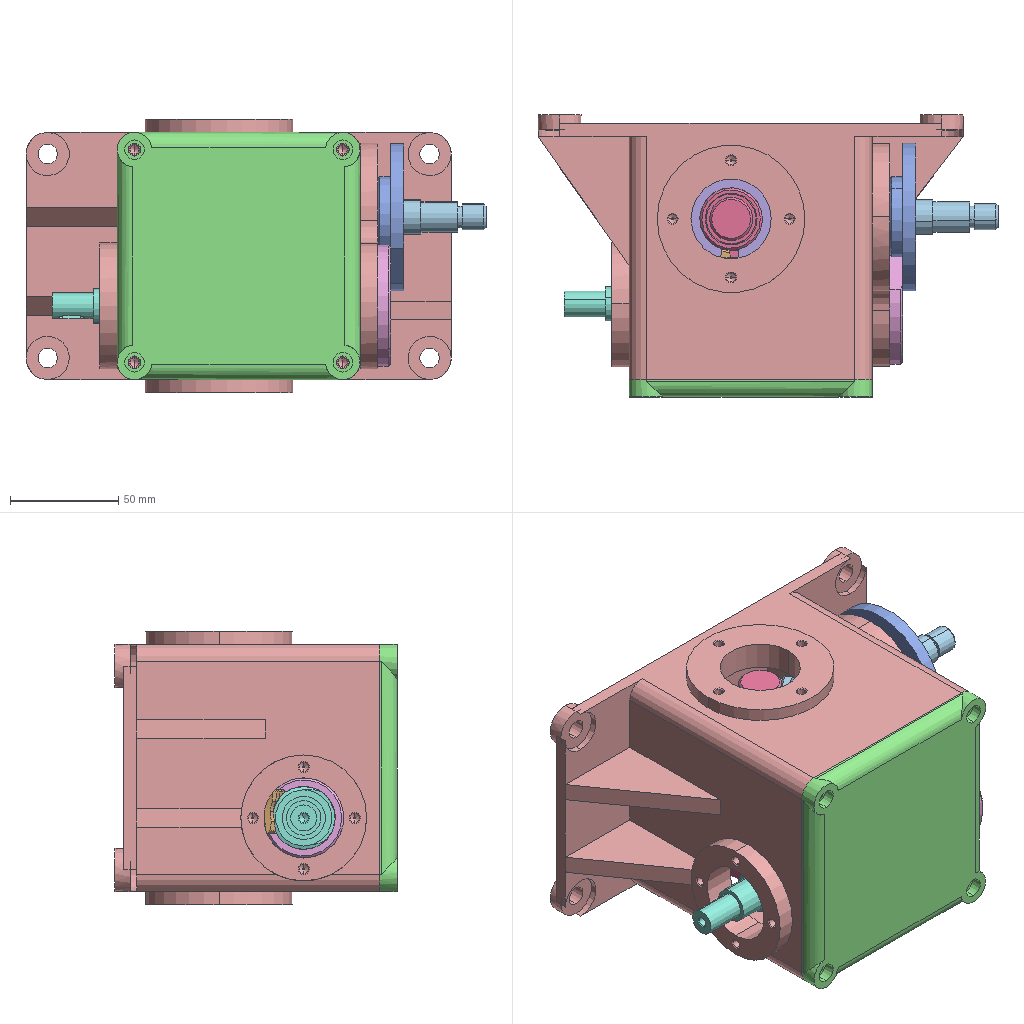Assembly | SolidWorks | 10 different items | 10 placed | box 212 x 130 x 126 mm
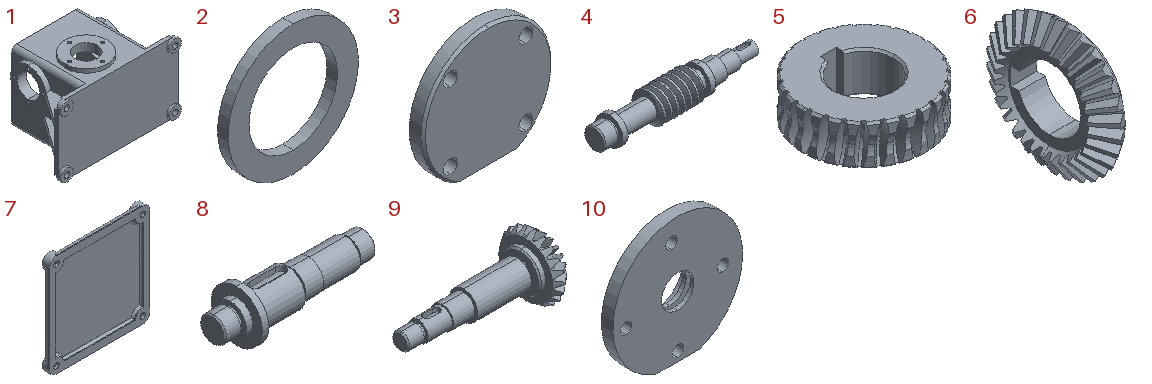Parts list (item | quantity | size | volume | features):
1 | x1 | 196 x 122 x 126 mm | 549396 mm3 | features ICE 13, HoleWzd 5, MirrorPattern 3, Rib 3, DelFace 1, Extrusion 1, Revolution 1
2 | x1 | 25 x 2 x 25 mm | 527.788 mm3 | features Extrusion 1
3 | x1 | 56 x 12 x 52 mm | 16065 mm3 | features ICE 4, Chamfer 1, Extrusion 1, Fillet 1
4 | x1 | 150 x 29 x 29 mm | 48060 mm3 | features ICE 11, Chamfer 1, Extrusion 1, Helix 1, HoleWzd 1, SweepCut 1
5 | x1 | 61 x 60.994 x 20 mm | 37460 mm3 | features Chamfer 2, ICE 2, CirPattern 1, Extrusion 1, Helix 1, RevCut 1, SweepCut 1
6 | x1 | 16 x 62.135 x 62.3 mm | 17909 mm3 | features BlendCut 1, CirPattern 1, ICE 1, Revolution 1
7 | x1 | 112 x 8 x 114 mm | 68573 mm3 | features Fillet 2, ICE 2, Extrusion 1, HoleWzd 1
8 | x1 | 118 x 40 x 40 mm | 58470 mm3 | features ICE 11, Chamfer 1, Extrusion 1
9 | x1 | 102 x 45.084 x 45.195 mm | 33414 mm3 | features ICE 7, BlendCut 1, Chamfer 1, CirPattern 1, Extrusion 1, Revolution 1, StudWizard 1
10 | x1 | 68 x 12 x 66 mm | 21544 mm3 | features ICE 7, Chamfer 1, Extrusion 1, Fillet 1
Mates (type | each side: item.copy, entity, surface, feature):
Coincident | 1.1 plane | assembly plane | 3 times
Concentric | 1.1 face cylinder Cut-Extrude4 | 4.1 face cylinder Boss-Extrude4
Concentric | 1.1 face cylinder Cut-Extrude6 | 8.1 face cylinder Boss-Extrude9
Concentric | 6.1 face cylinder Revolve1 | 8.1 face cylinder Boss-Extrude6
Concentric | 10.1 face cylinder Boss-Extrude1 | assembly face
Concentric | 10.1 face cylinder Cut-Extrude6 | assembly face
Coincident | 10.1 face plane Boss-Extrude1 | assembly face
Concentric | 1.1 face cylinder Mirror3 | assembly face | 2 times
Coincident | 1.1 face plane Mirror3 | assembly face
Concentric | 1.1 face cylinder Cut-Extrude6 | assembly face
Concentric | 1.1 face cylinder M5 Tapped Hole5 | assembly face
Coincident | 1.1 face plane Boss-Extrude6 | assembly face
Concentric | 1.1 face cylinder Cut-Extrude5 | assembly face
Concentric | 5.1 face cylinder Cut-Extrude1 | 8.1 face cylinder Boss-Extrude9
Parallel | 5.1 face plane Cut-Extrude2 | 8.1 face plane Cut-Extrude1
Coincident | 1.1 face plane Boss-Extrude4 | assembly face
Concentric | 1.1 face cylinder M5 Tapped Hole3 | assembly face
Concentric | 1.1 face cylinder Cut-Extrude4 | 3.1 face cylinder Cut-Extrude1
Concentric | 1.1 face cylinder M5 Tapped Hole2 | 3.1 face cylinder Cut-Extrude2
Coincident | 1.1 face plane Boss-Extrude4 | 3.1 face plane Boss-Extrude1
Concentric | 1.1 face cylinder Cut-Extrude4 | assembly face
Concentric | 1.1 face cylinder M5 Tapped Hole4 | assembly face
Coincident | 1.1 face plane Boss-Extrude5 | assembly face
Coincident | 1.1 face plane Boss-Extrude3 | 7.1 face plane Boss-Extrude1 | 2 times
Concentric | 1.1 face cylinder M5 Tapped Hole1 | 7.1 face cylinder Hole2
Coincident | 5.1 face plane Boss-Extrude1 | 8.1 edge
Coincident | assembly face | 8.1 face plane Boss-Extrude1
Concentric | 10.1 face cylinder Cut-Extrude4 | 9.1 face cylinder Boss-Extrude1
Coincident | 9.1 face plane Boss-Extrude5 | assembly face
Concentric | assembly face | 8.1 face cylinder Boss-Extrude6
Coincident | 5.1 face plane Boss-Extrude1 | assembly face
Coincident | 5.1 face plane Cut-Extrude2 | assembly face
Concentric | 2.1 face cylinder Boss-Extrude1 | 9.1 face cylinder Boss-Extrude3
Concentric | 9.1 face cylinder Boss-Extrude1 | assembly face
Concentric | 9.1 face cylinder Boss-Extrude3 | assembly face
Coincident | 10.1 face plane Cut-Extrude3 | 2.1 face plane Boss-Extrude1
Coincident | 10.1 face plane Cut-Extrude1 | assembly face
Coincident | assembly face | assembly face
Coincident | 5.1 face plane Boss-Extrude1 | 6.1 face plane Revolve1
Coincident | 1.1 face plane Boss-Extrude4 | 4.1 edge